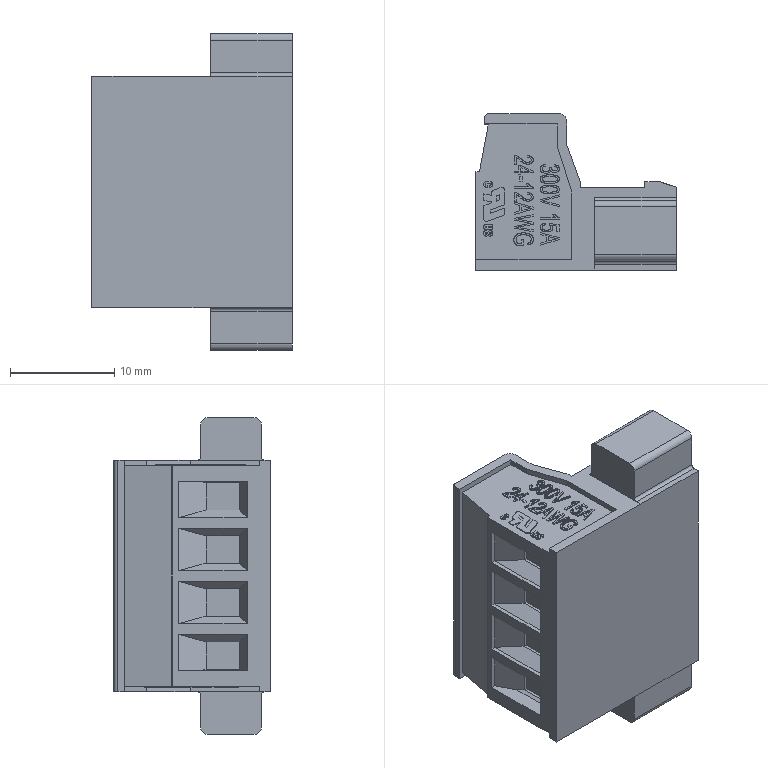Part | NX | features BREP 11 | 11 solids | 3789 faces | volume 3758 mm3 | plane 3465 | cylinder 160 | spline 116 | torus 32 | cone 16 | commonest cylinder face diameters 3.2 x40 3.6 x36 3.9 x8 4 x8 0.677 x6 0.146 x4